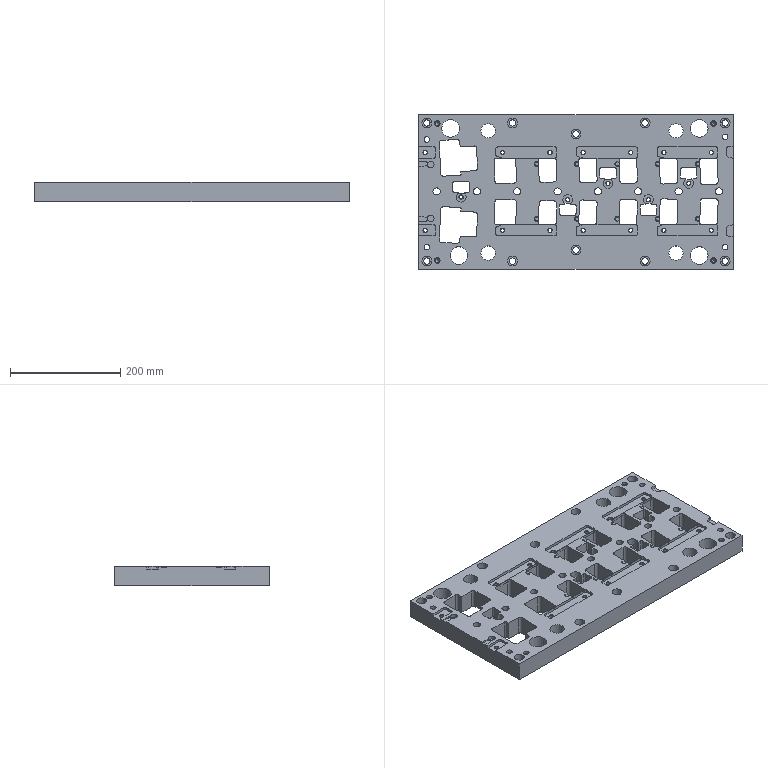Part | NX | features DIE-46 2 | 1 solid | 550 faces | box 570 x 280 x 35.001 mm | volume 4163611 mm3 | cylinder 246 | plane 229 | spline 52 | cone 23 | commonest cylinder face diameters 6 x54 10 x28 18 x23 1 x20 2 x20 5 x14